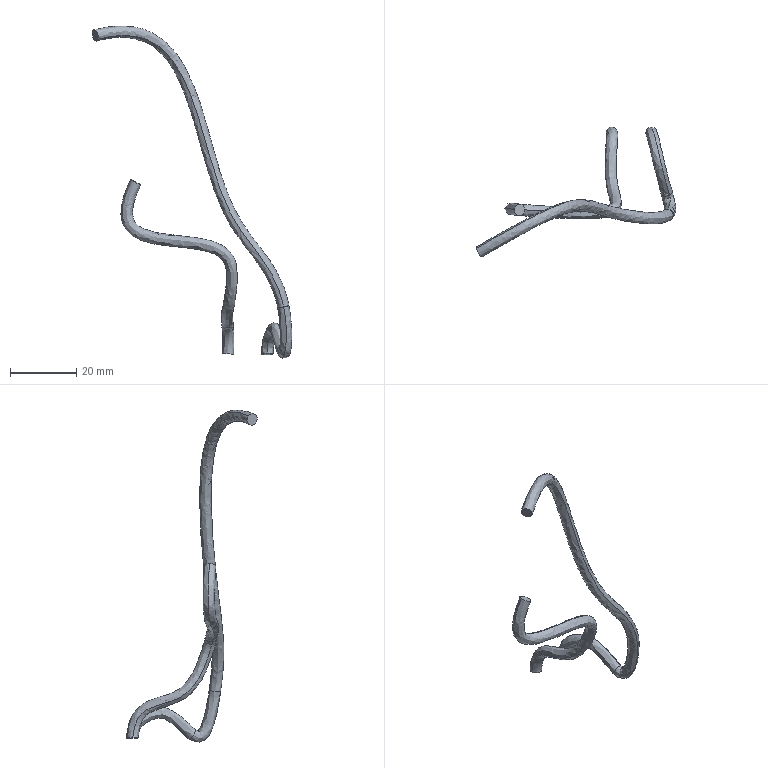Part | SolidWorks | features BaseBody 2 | 2 solids | 12 faces | box 60.243 x 39.383 x 100.293 mm | volume 2315 mm3 | spline 8 | plane 4